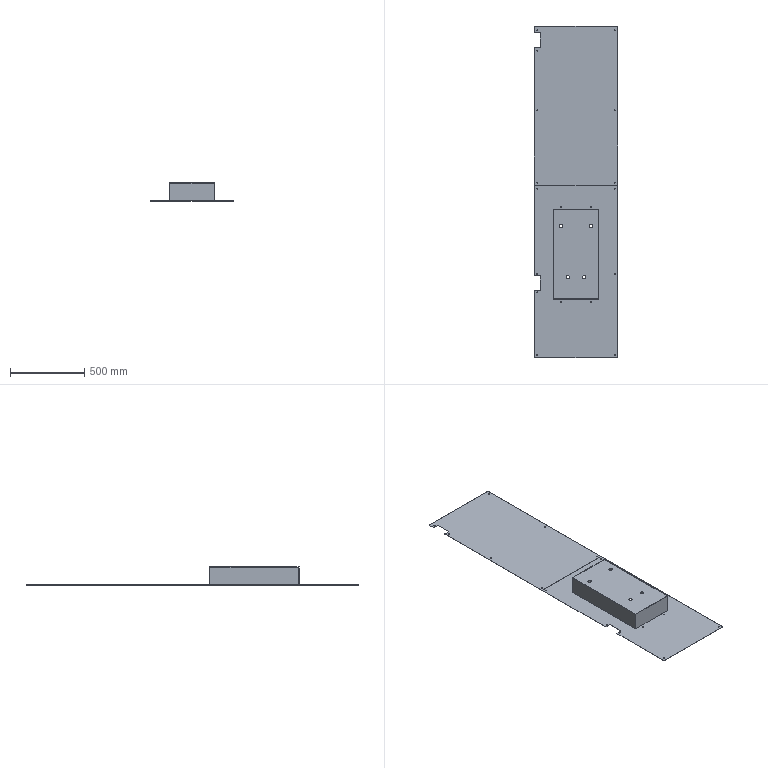Part | SolidWorks | features ICE 7, Fillet 4, HoleWzd 3, FlatPattern 2, SMBaseFlange 1, SheetMetal 1 | 2 solids | 90 faces | box 560 x 2240 x 122 mm | volume 2071529 mm3 | cylinder 60 | plane 30 | commonest cylinder face diameters 7 x28 6 x16 5.3 x8 22 x8